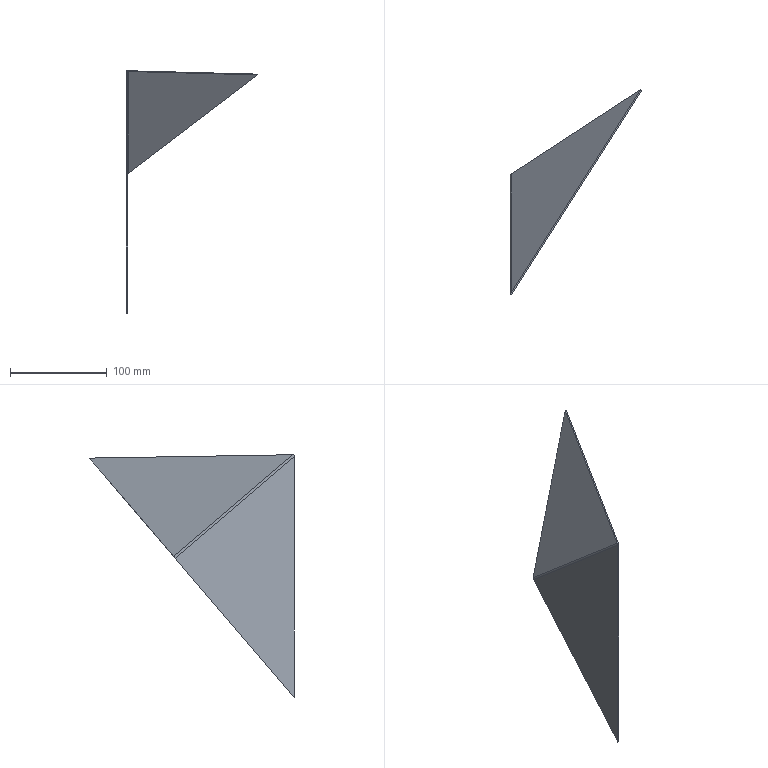Part | SolidWorks | features BaseBody 1 | 1 solid | 11 faces | box 135.69 x 211.419 x 250.496 mm | volume 46324 mm3 | plane 7 | cylinder 2 | spline 2 | commonest cylinder face diameters 3 x1 6 x1
STEP:
#1=CARTESIAN_POINT('',(1.5,0.,248.884));
#2=VERTEX_POINT('',#1);
#3=CARTESIAN_POINT('',(1.5,0.,0.));
#4=VERTEX_POINT('',#3);
#5=CARTESIAN_POINT('',(1.5,0.,174.4));
#6=DIRECTION('',(0.,0.,-1.));
#7=VECTOR('',#6,1000.);
#8=LINE('',#5,#7);
#9=EDGE_CURVE('',#2,#4,#8,.T.);
#10=ORIENTED_EDGE('',*,*,#9,.T.);
#11=CARTESIAN_POINT('',(1.5,122.934,143.755));
#12=VERTEX_POINT('',#11);
#13=CARTESIAN_POINT('',(1.5,0.,0.));
#14=DIRECTION('',(0.,0.6499,0.76));
#15=VECTOR('',#14,1000.);
#16=LINE('',#13,#15);
#17=EDGE_CURVE('',#4,#12,#16,.T.);
#18=ORIENTED_EDGE('',*,*,#17,.T.);
#19=CARTESIAN_POINT('',(1.5,122.934,143.755));
#20=DIRECTION('',(0.,-0.76,0.6499));
#21=VECTOR('',#20,1000.);
#22=LINE('',#19,#21);
#23=EDGE_CURVE('',#12,#2,#22,.T.);
#24=ORIENTED_EDGE('',*,*,#23,.T.);
#25=EDGE_LOOP('',(#10,#18,#24));
#26=FACE_OUTER_BOUND('',#25,.T.);
#27=CARTESIAN_POINT('',(1.5,88.404,174.4));
#28=DIRECTION('',(1.,0.,0.));
#29=DIRECTION('',(0.,0.,-1.));
#30=AXIS2_PLACEMENT_3D('',#27,#28,#29);
#31=PLANE('',#30);
#32=ADVANCED_FACE('',(#26),#31,.T.);
#33=CARTESIAN_POINT('',(0.,0.,0.));
#34=VERTEX_POINT('',#33);
#35=CARTESIAN_POINT('',(0.,0.,0.));
#36=DIRECTION('',(-1.,0.,0.));
#37=VECTOR('',#36,1000.);
#38=LINE('',#35,#37);
#39=EDGE_CURVE('',#4,#34,#38,.T.);
#40=ORIENTED_EDGE('',*,*,#39,.T.);
#41=CARTESIAN_POINT('',(0.,122.934,143.755));
#42=VERTEX_POINT('',#41);
#43=CARTESIAN_POINT('',(0.,246.971,288.8));
#44=DIRECTION('',(0.,0.6499,0.76));
#45=VECTOR('',#44,1000.);
#46=LINE('',#43,#45);
#47=EDGE_CURVE('',#34,#42,#46,.T.);
#48=ORIENTED_EDGE('',*,*,#47,.T.);
#49=CARTESIAN_POINT('',(0.8787,124.313,145.368));
#50=VERTEX_POINT('',#49);
#51=CARTESIAN_POINT('',(3.,122.934,143.755));
#52=DIRECTION('',(0.,-0.76,0.6499));
#53=DIRECTION('',(0.,0.6499,0.76));
#54=AXIS2_PLACEMENT_3D('',#51,#52,#53);
#55=CIRCLE('',#54,3.);
#56=EDGE_CURVE('',#50,#42,#55,.T.);
#57=ORIENTED_EDGE('',*,*,#56,.F.);
#58=CARTESIAN_POINT('',(134.629,211.24,247.018));
#59=VERTEX_POINT('',#58);
#60=CARTESIAN_POINT('',(0.8787,124.313,145.368));
#61=DIRECTION('',(0.7071,0.4596,0.5374));
#62=VECTOR('',#61,1000.);
#63=LINE('',#60,#62);
#64=EDGE_CURVE('',#50,#59,#63,.T.);
#65=ORIENTED_EDGE('',*,*,#64,.T.);
#66=CARTESIAN_POINT('',(135.69,210.551,246.212));
#67=VERTEX_POINT('',#66);
#68=CARTESIAN_POINT('',(135.69,210.551,246.212));
#69=DIRECTION('',(-0.7071,0.4596,0.5374));
#70=VECTOR('',#69,1000.);
#71=LINE('',#68,#70);
#72=EDGE_CURVE('',#67,#59,#71,.T.);
#73=ORIENTED_EDGE('',*,*,#72,.F.);
#74=CARTESIAN_POINT('',(1.939,123.623,144.561));
#75=VERTEX_POINT('',#74);
#76=CARTESIAN_POINT('',(1.939,123.623,144.561));
#77=DIRECTION('',(0.7071,0.4596,0.5374));
#78=VECTOR('',#77,1000.);
#79=LINE('',#76,#78);
#80=EDGE_CURVE('',#75,#67,#79,.T.);
#81=ORIENTED_EDGE('',*,*,#80,.F.);
#82=CARTESIAN_POINT('',(3.,122.934,143.755));
#83=DIRECTION('',(0.,0.76,-0.6499));
#84=DIRECTION('',(0.,0.6499,0.76));
#85=AXIS2_PLACEMENT_3D('',#82,#83,#84);
#86=CIRCLE('',#85,1.5);
#87=EDGE_CURVE('',#12,#75,#86,.T.);
#88=ORIENTED_EDGE('',*,*,#87,.F.);
#89=ORIENTED_EDGE('',*,*,#17,.F.);
#90=EDGE_LOOP('',(#40,#48,#57,#65,#73,#81,#88,#89));
#91=FACE_OUTER_BOUND('',#90,.T.);
#92=CARTESIAN_POINT('',(0.,246.971,288.8));
#93=DIRECTION('',(0.,0.76,-0.6499));
#94=DIRECTION('',(0.,0.6499,0.76));
#95=AXIS2_PLACEMENT_3D('',#92,#93,#94);
#96=PLANE('',#95);
#97=ADVANCED_FACE('',(#91),#96,.T.);
#98=ORIENTED_EDGE('',*,*,#39,.F.);
#99=ORIENTED_EDGE('',*,*,#9,.F.);
#100=CARTESIAN_POINT('',(0.,0.,248.884));
#101=VERTEX_POINT('',#100);
#102=CARTESIAN_POINT('',(0.,0.,248.884));
#103=DIRECTION('',(-1.,0.,0.));
#104=VECTOR('',#103,1000.);
#105=LINE('',#102,#104);
#106=EDGE_CURVE('',#2,#101,#105,.T.);
#107=ORIENTED_EDGE('',*,*,#106,.T.);
#108=CARTESIAN_POINT('',(0.,0.,0.));
#109=DIRECTION('',(0.,0.,-1.));
#110=VECTOR('',#109,1000.);
#111=LINE('',#108,#110);
#112=EDGE_CURVE('',#101,#34,#111,.T.);
#113=ORIENTED_EDGE('',*,*,#112,.T.);
#114=EDGE_LOOP('',(#98,#99,#107,#113));
#115=FACE_OUTER_BOUND('',#114,.T.);
#116=CARTESIAN_POINT('',(0.,0.,0.));
#117=DIRECTION('',(0.,-1.,0.));
#118=DIRECTION('',(0.,0.,-1.));
#119=AXIS2_PLACEMENT_3D('',#116,#117,#118);
#120=PLANE('',#119);
#121=ADVANCED_FACE('',(#115),#120,.T.);
#122=ORIENTED_EDGE('',*,*,#23,.F.);
#123=ORIENTED_EDGE('',*,*,#87,.T.);
#124=CARTESIAN_POINT('',(1.939,0.6893,249.69));
#125=VERTEX_POINT('',#124);
#126=CARTESIAN_POINT('',(1.939,62.156,197.126));
#127=DIRECTION('',(0.,0.76,-0.6499));
#128=VECTOR('',#127,1000.);
#129=LINE('',#126,#128);
#130=EDGE_CURVE('',#125,#75,#129,.T.);
#131=ORIENTED_EDGE('',*,*,#130,.F.);
#132=CARTESIAN_POINT('',(1.614,-0.1782,249.792));
#133=VERTEX_POINT('',#132);
#134=CARTESIAN_POINT('',(1.614,-0.1782,249.792));
#135=CARTESIAN_POINT('',(1.689,0.1234,249.772));
#136=CARTESIAN_POINT('',(1.8,0.4154,249.742));
#137=CARTESIAN_POINT('',(1.939,0.6893,249.69));
#138=B_SPLINE_CURVE_WITH_KNOTS('',3,(#134,#135,#136,#137),.UNSPECIFIED.,.F.,.F.,(4,4),(0.,1.),.UNSPECIFIED.);
#139=EDGE_CURVE('',#133,#125,#138,.T.);
#140=ORIENTED_EDGE('',*,*,#139,.F.);
#141=CARTESIAN_POINT('',(1.5,0.,248.884));
#142=CARTESIAN_POINT('',(1.5,-0.05615,249.19));
#143=CARTESIAN_POINT('',(1.539,-0.1123,249.497));
#144=CARTESIAN_POINT('',(1.614,-0.1782,249.792));
#145=B_SPLINE_CURVE_WITH_KNOTS('',3,(#141,#142,#143,#144),.UNSPECIFIED.,.F.,.F.,(4,4),(0.,1.),.UNSPECIFIED.);
#146=EDGE_CURVE('',#2,#133,#145,.T.);
#147=ORIENTED_EDGE('',*,*,#146,.F.);
#148=EDGE_LOOP('',(#122,#123,#131,#140,#147));
#149=FACE_OUTER_BOUND('',#148,.T.);
#150=CARTESIAN_POINT('',(3.,61.467,196.32));
#151=DIRECTION('',(0.,0.76,-0.6499));
#152=DIRECTION('',(0.,0.6499,0.76));
#153=AXIS2_PLACEMENT_3D('',#150,#151,#152);
#154=CYLINDRICAL_SURFACE('',#153,1.5);
#155=ADVANCED_FACE('',(#149),#154,.F.);
#156=ORIENTED_EDGE('',*,*,#47,.F.);
#157=ORIENTED_EDGE('',*,*,#112,.F.);
#158=CARTESIAN_POINT('',(0.,122.934,143.755));
#159=DIRECTION('',(0.,-0.76,0.6499));
#160=VECTOR('',#159,1000.);
#161=LINE('',#158,#160);
#162=EDGE_CURVE('',#42,#101,#161,.T.);
#163=ORIENTED_EDGE('',*,*,#162,.F.);
#164=EDGE_LOOP('',(#156,#157,#163));
#165=FACE_OUTER_BOUND('',#164,.T.);
#166=CARTESIAN_POINT('',(0.,88.404,174.4));
#167=DIRECTION('',(1.,0.,0.));
#168=DIRECTION('',(0.,0.,-1.));
#169=AXIS2_PLACEMENT_3D('',#166,#167,#168);
#170=PLANE('',#169);
#171=ADVANCED_FACE('',(#165),#170,.F.);
#172=ORIENTED_EDGE('',*,*,#106,.F.);
#173=ORIENTED_EDGE('',*,*,#146,.T.);
#174=CARTESIAN_POINT('',(0.2284,0.1949,250.228));
#175=VERTEX_POINT('',#174);
#176=CARTESIAN_POINT('',(-2.197,0.8477,250.991));
#177=DIRECTION('',(0.9239,-0.2487,-0.2908));
#178=VECTOR('',#177,1000.);
#179=LINE('',#176,#178);
#180=EDGE_CURVE('',#175,#133,#179,.T.);
#181=ORIENTED_EDGE('',*,*,#180,.F.);
#182=CARTESIAN_POINT('',(0.,0.,248.884));
#183=CARTESIAN_POINT('',(0.,0.07146,249.34));
#184=CARTESIAN_POINT('',(0.07808,0.1428,249.795));
#185=CARTESIAN_POINT('',(0.2284,0.1949,250.228));
#186=B_SPLINE_CURVE_WITH_KNOTS('',3,(#182,#183,#184,#185),.UNSPECIFIED.,.F.,.F.,(4,4),(0.,1.),.UNSPECIFIED.);
#187=EDGE_CURVE('',#101,#175,#186,.T.);
#188=ORIENTED_EDGE('',*,*,#187,.F.);
#189=EDGE_LOOP('',(#172,#173,#181,#188));
#190=FACE_OUTER_BOUND('',#189,.T.);
#191=CARTESIAN_POINT('',(2.25,0.,248.884));
#192=CARTESIAN_POINT('',(2.25,-0.008568,248.9));
#193=CARTESIAN_POINT('',(2.25,-0.0257,248.934));
#194=CARTESIAN_POINT('',(2.251,-0.05142,248.983));
#195=CARTESIAN_POINT('',(2.253,-0.07716,249.033));
#196=CARTESIAN_POINT('',(2.255,-0.1029,249.082));
#197=CARTESIAN_POINT('',(2.257,-0.1287,249.132));
#198=CARTESIAN_POINT('',(2.26,-0.1546,249.181));
#199=CARTESIAN_POINT('',(2.264,-0.1805,249.231));
#200=CARTESIAN_POINT('',(2.269,-0.2065,249.28));
#201=CARTESIAN_POINT('',(2.274,-0.2326,249.329));
#202=CARTESIAN_POINT('',(2.279,-0.2588,249.378));
#203=CARTESIAN_POINT('',(2.285,-0.2851,249.427));
#204=CARTESIAN_POINT('',(2.292,-0.3115,249.476));
#205=CARTESIAN_POINT('',(2.299,-0.3381,249.525));
#206=CARTESIAN_POINT('',(2.304,-0.3558,249.557));
#207=CARTESIAN_POINT('',(2.307,-0.3647,249.573));
#208=CARTESIAN_POINT('',(1.78,0.,248.884));
#209=CARTESIAN_POINT('',(1.78,-0.005712,248.904));
#210=CARTESIAN_POINT('',(1.78,-0.01714,248.944));
#211=CARTESIAN_POINT('',(1.782,-0.03429,249.003));
#212=CARTESIAN_POINT('',(1.784,-0.05148,249.063));
#213=CARTESIAN_POINT('',(1.788,-0.06872,249.122));
#214=CARTESIAN_POINT('',(1.792,-0.08603,249.182));
#215=CARTESIAN_POINT('',(1.797,-0.1034,249.241));
#216=CARTESIAN_POINT('',(1.803,-0.1209,249.301));
#217=CARTESIAN_POINT('',(1.81,-0.1386,249.36));
#218=CARTESIAN_POINT('',(1.819,-0.1563,249.419));
#219=CARTESIAN_POINT('',(1.828,-0.1742,249.477));
#220=CARTESIAN_POINT('',(1.837,-0.1923,249.536));
#221=CARTESIAN_POINT('',(1.848,-0.2106,249.594));
#222=CARTESIAN_POINT('',(1.86,-0.2291,249.652));
#223=CARTESIAN_POINT('',(1.869,-0.2416,249.691));
#224=CARTESIAN_POINT('',(1.873,-0.2479,249.71));
#225=CARTESIAN_POINT('',(-1.47,0.,248.884));
#226=CARTESIAN_POINT('',(-1.47,0.01404,248.927));
#227=CARTESIAN_POINT('',(-1.469,0.04211,249.013));
#228=CARTESIAN_POINT('',(-1.464,0.08416,249.142));
#229=CARTESIAN_POINT('',(-1.455,0.1261,249.271));
#230=CARTESIAN_POINT('',(-1.442,0.1678,249.399));
#231=CARTESIAN_POINT('',(-1.427,0.2093,249.527));
#232=CARTESIAN_POINT('',(-1.407,0.2504,249.655));
#233=CARTESIAN_POINT('',(-1.385,0.2912,249.782));
#234=CARTESIAN_POINT('',(-1.358,0.3315,249.909));
#235=CARTESIAN_POINT('',(-1.329,0.3713,250.036));
#236=CARTESIAN_POINT('',(-1.296,0.4106,250.161));
#237=CARTESIAN_POINT('',(-1.259,0.4492,250.286));
#238=CARTESIAN_POINT('',(-1.22,0.4871,250.41));
#239=CARTESIAN_POINT('',(-1.177,0.5243,250.533));
#240=CARTESIAN_POINT('',(-1.146,0.5485,250.615));
#241=CARTESIAN_POINT('',(-1.13,0.5605,250.655));
#242=CARTESIAN_POINT('',(-4.72,0.,248.884));
#243=CARTESIAN_POINT('',(-4.72,0.03379,248.95));
#244=CARTESIAN_POINT('',(-4.718,0.1014,249.082));
#245=CARTESIAN_POINT('',(-4.709,0.2026,249.28));
#246=CARTESIAN_POINT('',(-4.694,0.3036,249.478));
#247=CARTESIAN_POINT('',(-4.672,0.4043,249.676));
#248=CARTESIAN_POINT('',(-4.645,0.5046,249.873));
#249=CARTESIAN_POINT('',(-4.612,0.6043,250.069));
#250=CARTESIAN_POINT('',(-4.573,0.7033,250.264));
#251=CARTESIAN_POINT('',(-4.527,0.8016,250.459));
#252=CARTESIAN_POINT('',(-4.476,0.899,250.653));
#253=CARTESIAN_POINT('',(-4.419,0.9954,250.845));
#254=CARTESIAN_POINT('',(-4.356,1.091,251.036));
#255=CARTESIAN_POINT('',(-4.288,1.185,251.226));
#256=CARTESIAN_POINT('',(-4.213,1.278,251.414));
#257=CARTESIAN_POINT('',(-4.16,1.339,251.539));
#258=CARTESIAN_POINT('',(-4.132,1.369,251.601));
#259=CARTESIAN_POINT('',(-7.5,0.,248.884));
#260=CARTESIAN_POINT('',(-7.5,0.05068,248.97));
#261=CARTESIAN_POINT('',(-7.497,0.152,249.141));
#262=CARTESIAN_POINT('',(-7.485,0.3039,249.399));
#263=CARTESIAN_POINT('',(-7.464,0.4555,249.656));
#264=CARTESIAN_POINT('',(-7.435,0.6067,249.912));
#265=CARTESIAN_POINT('',(-7.398,0.7572,250.168));
#266=CARTESIAN_POINT('',(-7.353,0.907,250.423));
#267=CARTESIAN_POINT('',(-7.3,1.056,250.677));
#268=CARTESIAN_POINT('',(-7.238,1.204,250.929));
#269=CARTESIAN_POINT('',(-7.169,1.35,251.18));
#270=CARTESIAN_POINT('',(-7.091,1.496,251.43));
#271=CARTESIAN_POINT('',(-7.005,1.639,251.678));
#272=CARTESIAN_POINT('',(-6.912,1.782,251.924));
#273=CARTESIAN_POINT('',(-6.811,1.922,252.168));
#274=CARTESIAN_POINT('',(-6.738,2.014,252.329));
#275=CARTESIAN_POINT('',(-6.701,2.06,252.409));
#276=B_SPLINE_SURFACE_WITH_KNOTS('',3,3,((#191,#192,#193,#194,#195,#196,#197,#198,#199,#200,#201,#202,#203,#204,#205,#206,#207),(#208,#209,#210,#211,#212,#213,#214,#215,#216,#217,#218,#219,#220,#221,#222,#223,#224),(#225,#226,#227,#228,#229,#230,#231,#232,#233,#234,#235,#236,#237,#238,#239,#240,#241),(#242,#243,#244,#245,#246,#247,#248,#249,#250,#251,#252,#253,#254,#255,#256,#257,#258),(#259,#260,#261,#262,#263,#264,#265,#266,#267,#268,#269,#270,#271,#272,#273,#274,#275)),.UNSPECIFIED.,.F.,.F.,.F.,(4,1,4),(4,1,1,1,1,1,1,1,1,1,1,1,1,1,4),(0.,0.141,0.975),(0.,0.01551,0.03101,0.04652,0.06203,0.07754,0.09304,0.1086,0.1241,0.1396,0.1551,0.1706,0.1861,0.2016,0.2171),.UNSPECIFIED.);
#277=ADVANCED_FACE('',(#190),#276,.F.);
#278=ORIENTED_EDGE('',*,*,#80,.T.);
#279=CARTESIAN_POINT('',(135.69,210.551,246.212));
#280=DIRECTION('',(-0.5374,-0.8432,0.01398));
#281=VECTOR('',#280,1000.);
#282=LINE('',#279,#281);
#283=EDGE_CURVE('',#67,#125,#282,.T.);
#284=ORIENTED_EDGE('',*,*,#283,.T.);
#285=ORIENTED_EDGE('',*,*,#130,.T.);
#286=EDGE_LOOP('',(#278,#284,#285));
#287=FACE_OUTER_BOUND('',#286,.T.);
#288=CARTESIAN_POINT('',(1.34,88.153,174.106));
#289=DIRECTION('',(0.7071,-0.4596,-0.5374));
#290=DIRECTION('',(-0.6051,0.,-0.7962));
#291=AXIS2_PLACEMENT_3D('',#288,#289,#290);
#292=PLANE('',#291);
#293=ADVANCED_FACE('',(#287),#292,.T.);
#294=ORIENTED_EDGE('',*,*,#180,.T.);
#295=ORIENTED_EDGE('',*,*,#139,.T.);
#296=CARTESIAN_POINT('',(0.8787,1.379,250.496));
#297=VERTEX_POINT('',#296);
#298=CARTESIAN_POINT('',(-0.9775,2.585,251.907));
#299=DIRECTION('',(0.7071,-0.4596,-0.5374));
#300=VECTOR('',#299,1000.);
#301=LINE('',#298,#300);
#302=EDGE_CURVE('',#297,#125,#301,.T.);
#303=ORIENTED_EDGE('',*,*,#302,.F.);
#304=CARTESIAN_POINT('',(0.2284,0.1949,250.228));
#305=CARTESIAN_POINT('',(0.3786,0.6144,250.346));
#306=CARTESIAN_POINT('',(0.601,1.014,250.442));
#307=CARTESIAN_POINT('',(0.8787,1.379,250.496));
#308=B_SPLINE_CURVE_WITH_KNOTS('',3,(#304,#305,#306,#307),.UNSPECIFIED.,.F.,.F.,(4,4),(0.000000345,1.),.UNSPECIFIED.);
#309=EDGE_CURVE('',#175,#297,#308,.T.);
#310=ORIENTED_EDGE('',*,*,#309,.F.);
#311=EDGE_LOOP('',(#294,#295,#303,#310));
#312=FACE_OUTER_BOUND('',#311,.T.);
#313=CARTESIAN_POINT('',(2.307,-0.3647,249.573));
#314=CARTESIAN_POINT('',(2.31,-0.3474,249.567));
#315=CARTESIAN_POINT('',(2.315,-0.3128,249.555));
#316=CARTESIAN_POINT('',(2.324,-0.261,249.535));
#317=CARTESIAN_POINT('',(2.334,-0.2094,249.516));
#318=CARTESIAN_POINT('',(2.343,-0.158,249.496));
#319=CARTESIAN_POINT('',(2.354,-0.1067,249.477));
#320=CARTESIAN_POINT('',(2.365,-0.05565,249.457));
#321=CARTESIAN_POINT('',(2.376,-0.004798,249.436));
#322=CARTESIAN_POINT('',(2.388,0.04584,249.416));
#323=CARTESIAN_POINT('',(2.401,0.09626,249.395));
#324=CARTESIAN_POINT('',(2.414,0.1464,249.374));
#325=CARTESIAN_POINT('',(2.427,0.1964,249.353));
#326=CARTESIAN_POINT('',(2.441,0.2461,249.331));
#327=CARTESIAN_POINT('',(2.455,0.2955,249.309));
#328=CARTESIAN_POINT('',(2.465,0.3283,249.294));
#329=CARTESIAN_POINT('',(2.47,0.3447,249.287));
#330=CARTESIAN_POINT('',(1.873,-0.2479,249.71));
#331=CARTESIAN_POINT('',(1.877,-0.2279,249.707));
#332=CARTESIAN_POINT('',(1.886,-0.188,249.7));
#333=CARTESIAN_POINT('',(1.901,-0.1285,249.69));
#334=CARTESIAN_POINT('',(1.916,-0.06917,249.68));
#335=CARTESIAN_POINT('',(1.932,-0.01018,249.669));
#336=CARTESIAN_POINT('',(1.949,0.04851,249.658));
#337=CARTESIAN_POINT('',(1.967,0.1069,249.647));
#338=CARTESIAN_POINT('',(1.985,0.1649,249.635));
#339=CARTESIAN_POINT('',(2.005,0.2226,249.623));
#340=CARTESIAN_POINT('',(2.025,0.28,249.61));
#341=CARTESIAN_POINT('',(2.046,0.3369,249.597));
#342=CARTESIAN_POINT('',(2.068,0.3935,249.583));
#343=CARTESIAN_POINT('',(2.09,0.4497,249.569));
#344=CARTESIAN_POINT('',(2.113,0.5054,249.555));
#345=CARTESIAN_POINT('',(2.129,0.5423,249.545));
#346=CARTESIAN_POINT('',(2.137,0.5607,249.54));
#347=CARTESIAN_POINT('',(-1.13,0.5605,250.655));
#348=CARTESIAN_POINT('',(-1.114,0.5987,250.674));
#349=CARTESIAN_POINT('',(-1.081,0.6748,250.709));
#350=CARTESIAN_POINT('',(-1.028,0.7881,250.762));
#351=CARTESIAN_POINT('',(-0.9719,0.9004,250.814));
#352=CARTESIAN_POINT('',(-0.9128,1.012,250.864));
#353=CARTESIAN_POINT('',(-0.8506,1.122,250.913));
#354=CARTESIAN_POINT('',(-0.7854,1.231,250.961));
#355=CARTESIAN_POINT('',(-0.7172,1.339,251.007));
#356=CARTESIAN_POINT('',(-0.646,1.445,251.052));
#357=CARTESIAN_POINT('',(-0.572,1.55,251.095));
#358=CARTESIAN_POINT('',(-0.4952,1.654,251.137));
#359=CARTESIAN_POINT('',(-0.4157,1.756,251.177));
#360=CARTESIAN_POINT('',(-0.3335,1.857,251.215));
#361=CARTESIAN_POINT('',(-0.2486,1.957,251.252));
#362=CARTESIAN_POINT('',(-0.1903,2.022,251.275));
#363=CARTESIAN_POINT('',(-0.1608,2.054,251.286));
#364=CARTESIAN_POINT('',(-4.132,1.369,251.601));
#365=CARTESIAN_POINT('',(-4.105,1.425,251.64));
#366=CARTESIAN_POINT('',(-4.048,1.538,251.718));
#367=CARTESIAN_POINT('',(-3.956,1.705,251.834));
#368=CARTESIAN_POINT('',(-3.86,1.87,251.948));
#369=CARTESIAN_POINT('',(-3.758,2.034,252.059));
#370=CARTESIAN_POINT('',(-3.65,2.195,252.168));
#371=CARTESIAN_POINT('',(-3.538,2.355,252.275));
#372=CARTESIAN_POINT('',(-3.42,2.512,252.38));
#373=CARTESIAN_POINT('',(-3.297,2.668,252.482));
#374=CARTESIAN_POINT('',(-3.169,2.821,252.581));
#375=CARTESIAN_POINT('',(-3.037,2.971,252.677));
#376=CARTESIAN_POINT('',(-2.899,3.119,252.771));
#377=CARTESIAN_POINT('',(-2.757,3.265,252.861));
#378=CARTESIAN_POINT('',(-2.611,3.408,252.949));
#379=CARTESIAN_POINT('',(-2.51,3.502,253.005));
#380=CARTESIAN_POINT('',(-2.459,3.548,253.033));
#381=CARTESIAN_POINT('',(-6.701,2.06,252.409));
#382=CARTESIAN_POINT('',(-6.663,2.132,252.467));
#383=CARTESIAN_POINT('',(-6.585,2.276,252.581));
#384=CARTESIAN_POINT('',(-6.461,2.489,252.751));
#385=CARTESIAN_POINT('',(-6.33,2.699,252.917));
#386=CARTESIAN_POINT('',(-6.191,2.908,253.081));
#387=CARTESIAN_POINT('',(-6.045,3.113,253.242));
#388=CARTESIAN_POINT('',(-5.892,3.316,253.399));
#389=CARTESIAN_POINT('',(-5.732,3.516,253.554));
#390=CARTESIAN_POINT('',(-5.565,3.713,253.704));
#391=CARTESIAN_POINT('',(-5.391,3.907,253.851));
#392=CARTESIAN_POINT('',(-5.21,4.098,253.995));
#393=CARTESIAN_POINT('',(-5.023,4.285,254.134));
#394=CARTESIAN_POINT('',(-4.83,4.469,254.269));
#395=CARTESIAN_POINT('',(-4.631,4.649,254.401));
#396=CARTESIAN_POINT('',(-4.494,4.767,254.485));
#397=CARTESIAN_POINT('',(-4.425,4.825,254.527));
#398=B_SPLINE_SURFACE_WITH_KNOTS('',3,3,((#313,#314,#315,#316,#317,#318,#319,#320,#321,#322,#323,#324,#325,#326,#327,#328,#329),(#330,#331,#332,#333,#334,#335,#336,#337,#338,#339,#340,#341,#342,#343,#344,#345,#346),(#347,#348,#349,#350,#351,#352,#353,#354,#355,#356,#357,#358,#359,#360,#361,#362,#363),(#364,#365,#366,#367,#368,#369,#370,#371,#372,#373,#374,#375,#376,#377,#378,#379,#380),(#381,#382,#383,#384,#385,#386,#387,#388,#389,#390,#391,#392,#393,#394,#395,#396,#397)),.UNSPECIFIED.,.F.,.F.,.F.,(4,1,4),(4,1,1,1,1,1,1,1,1,1,1,1,1,1,4),(0.,0.141,0.975),(0.,0.01551,0.03101,0.04652,0.06203,0.07754,0.09304,0.1086,0.1241,0.1396,0.1551,0.1706,0.1861,0.2016,0.2171),.UNSPECIFIED.);
#399=ADVANCED_FACE('',(#312),#398,.F.);
#400=ORIENTED_EDGE('',*,*,#162,.T.);
#401=ORIENTED_EDGE('',*,*,#187,.T.);
#402=ORIENTED_EDGE('',*,*,#309,.T.);
#403=CARTESIAN_POINT('',(0.8787,62.846,197.932));
#404=DIRECTION('',(0.,0.76,-0.6499));
#405=VECTOR('',#404,1000.);
#406=LINE('',#403,#405);
#407=EDGE_CURVE('',#297,#50,#406,.T.);
#408=ORIENTED_EDGE('',*,*,#407,.T.);
#409=ORIENTED_EDGE('',*,*,#56,.T.);
#410=EDGE_LOOP('',(#400,#401,#402,#408,#409));
#411=FACE_OUTER_BOUND('',#410,.T.);
#412=CARTESIAN_POINT('',(3.,61.467,196.32));
#413=DIRECTION('',(0.,0.76,-0.6499));
#414=DIRECTION('',(0.,0.6499,0.76));
#415=AXIS2_PLACEMENT_3D('',#412,#413,#414);
#416=CYLINDRICAL_SURFACE('',#415,3.);
#417=ADVANCED_FACE('',(#411),#416,.T.);
#418=ORIENTED_EDGE('',*,*,#72,.T.);
#419=CARTESIAN_POINT('',(134.629,211.24,247.018));
#420=DIRECTION('',(-0.5374,-0.8432,0.01398));
#421=VECTOR('',#420,1000.);
#422=LINE('',#419,#421);
#423=EDGE_CURVE('',#59,#297,#422,.T.);
#424=ORIENTED_EDGE('',*,*,#423,.T.);
#425=ORIENTED_EDGE('',*,*,#302,.T.);
#426=ORIENTED_EDGE('',*,*,#283,.F.);
#427=EDGE_LOOP('',(#418,#424,#425,#426));
#428=FACE_OUTER_BOUND('',#427,.T.);
#429=CARTESIAN_POINT('',(0.2789,0.4376,250.512));
#430=DIRECTION('',(0.4596,-0.2789,0.8432));
#431=DIRECTION('',(0.8781,0.,-0.4786));
#432=AXIS2_PLACEMENT_3D('',#429,#430,#431);
#433=PLANE('',#432);
#434=ADVANCED_FACE('',(#428),#433,.T.);
#435=ORIENTED_EDGE('',*,*,#423,.F.);
#436=ORIENTED_EDGE('',*,*,#64,.F.);
#437=ORIENTED_EDGE('',*,*,#407,.F.);
#438=EDGE_LOOP('',(#435,#436,#437));
#439=FACE_OUTER_BOUND('',#438,.T.);
#440=CARTESIAN_POINT('',(0.2789,88.842,174.912));
#441=DIRECTION('',(0.7071,-0.4596,-0.5374));
#442=DIRECTION('',(-0.6051,0.,-0.7962));
#443=AXIS2_PLACEMENT_3D('',#440,#441,#442);
#444=PLANE('',#443);
#445=ADVANCED_FACE('',(#439),#444,.F.);
#446=CLOSED_SHELL('',(#32,#97,#121,#155,#171,#277,#293,#399,#417,#434,#445));
#447=MANIFOLD_SOLID_BREP('',#446);
#448=CARTESIAN_POINT('',(0.,0.,0.));
#449=DIRECTION('',(0.,0.,1.));
#450=DIRECTION('',(1.,0.,0.));
#451=AXIS2_PLACEMENT_3D('',#448,#449,#450);
#452=(LENGTH_UNIT()NAMED_UNIT(*)SI_UNIT(.MILLI.,.METRE.));
#453=UNCERTAINTY_MEASURE_WITH_UNIT(LENGTH_MEASURE(0.00001),#452,'','');
#454=(NAMED_UNIT(*)PLANE_ANGLE_UNIT()SI_UNIT($,.RADIAN.));
#455=(NAMED_UNIT(*)SI_UNIT($,.STERADIAN.)SOLID_ANGLE_UNIT());
#456=(GEOMETRIC_REPRESENTATION_CONTEXT(3)GLOBAL_UNCERTAINTY_ASSIGNED_CONTEXT((#453))GLOBAL_UNIT_ASSIGNED_CONTEXT((#452,#454,#455))REPRESENTATION_CONTEXT('',''));
#457=ADVANCED_BREP_SHAPE_REPRESENTATION('',(#447,#451),#456);